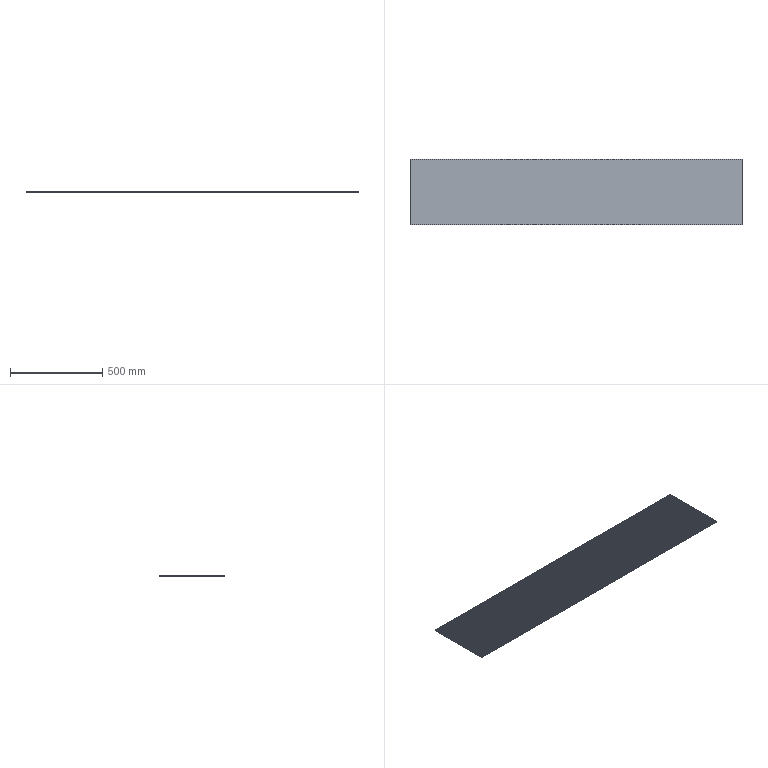Part | STEP file | 51E-01205JG10 | 1 solid | 954 faces | box 1800 x 355 x 5 mm | volume 1579291 mm3 | cylinder 947 | plane 7 | commonest cylinder face diameters 3.5 x947